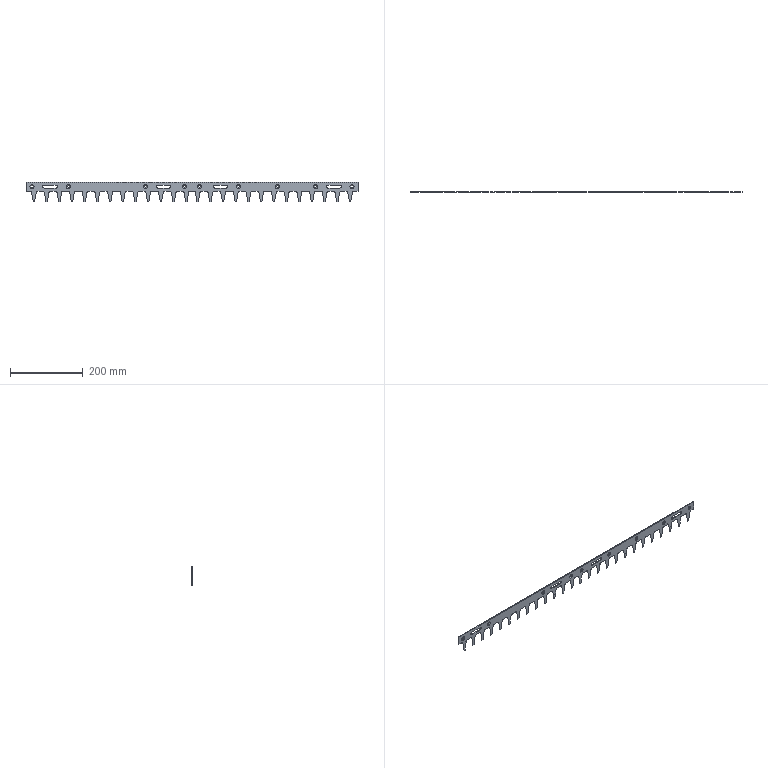Part | SolidWorks | features BaseBody 1, HoleWzd 1, ICE 1, MirrorSolid 1 | 1 solid | 196 faces | box 915 x 2.5 x 55 mm | volume 63974 mm3 | plane 118 | cone 70 | cylinder 8 | commonest cylinder face diameters 8 x8